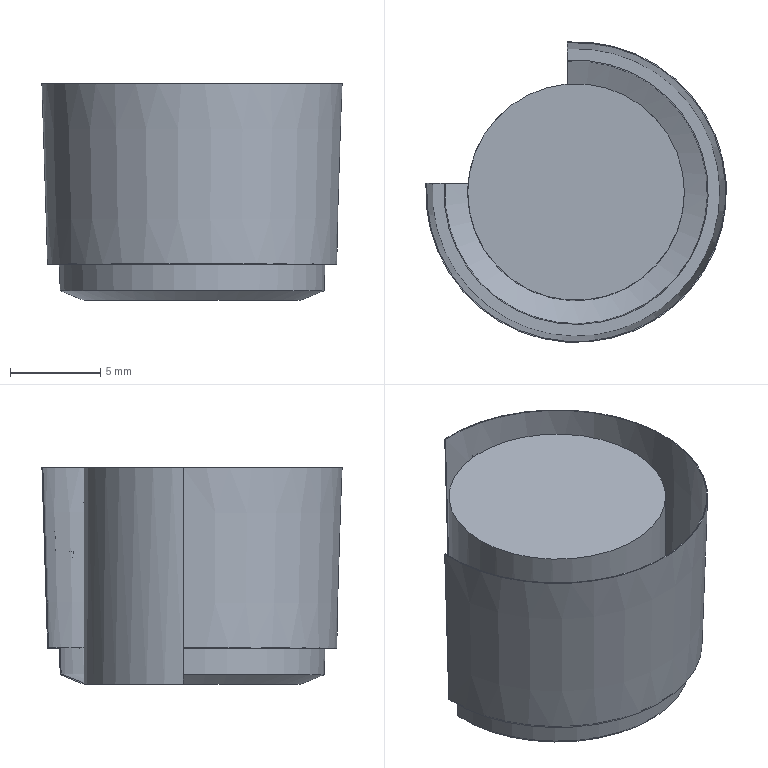Part | STEP file | SOLID | 1 solid | 57 faces | box 16.662 x 16.662 x 12.01 mm | volume 1384 mm3 | plane 26 | other 16 | cone 14 | cylinder 1 | commonest cylinder face diameters 12 x1